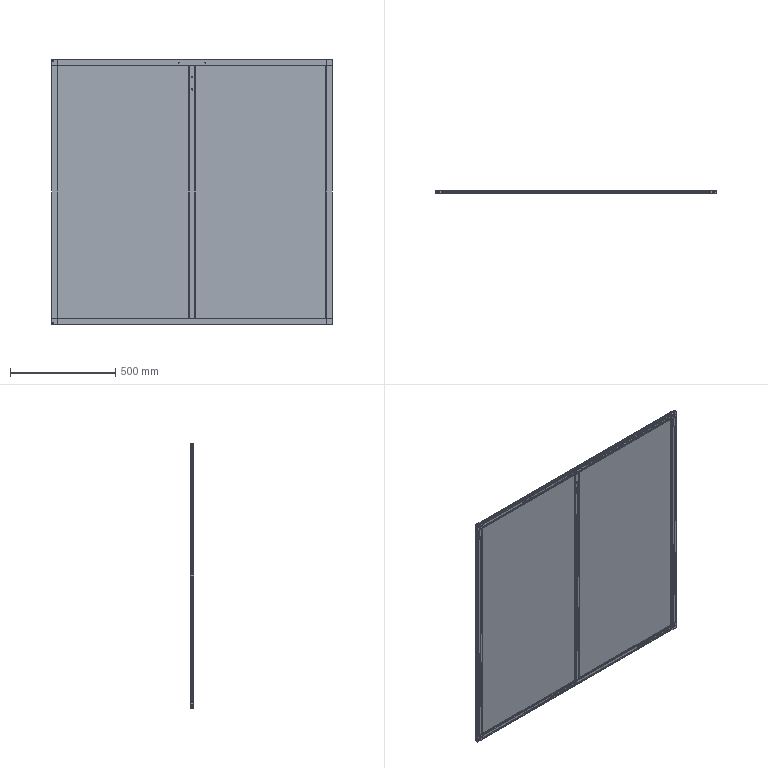Part | SolidWorks | features ReferencePattern 3, LocalLPattern 2 | 19 solids | 957 faces | box 1336 x 15 x 1260 mm | volume 9289979 mm3 | plane 578 | cylinder 275 | spline 52 | cone 52 | commonest cylinder face diameters 5 x89 11 x52 1 x42 2 x20 3.3 x16 4.5 x16